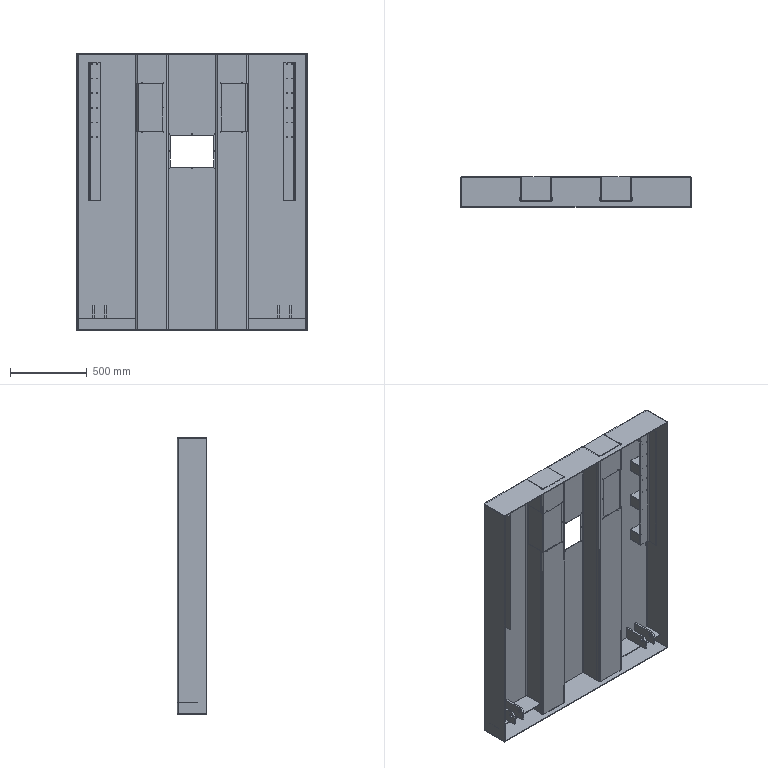Part | STEP file | PN_0001-01-01 Lifting platform top cover_Default<Machined> | 25 solids | 480 faces | box 1500 x 195 x 1800 mm | volume 133503358 mm3 | plane 250 | cylinder 230 | commonest cylinder face diameters 5 x96 4 x32 8 x32 10 x28 20 x28 25 x8